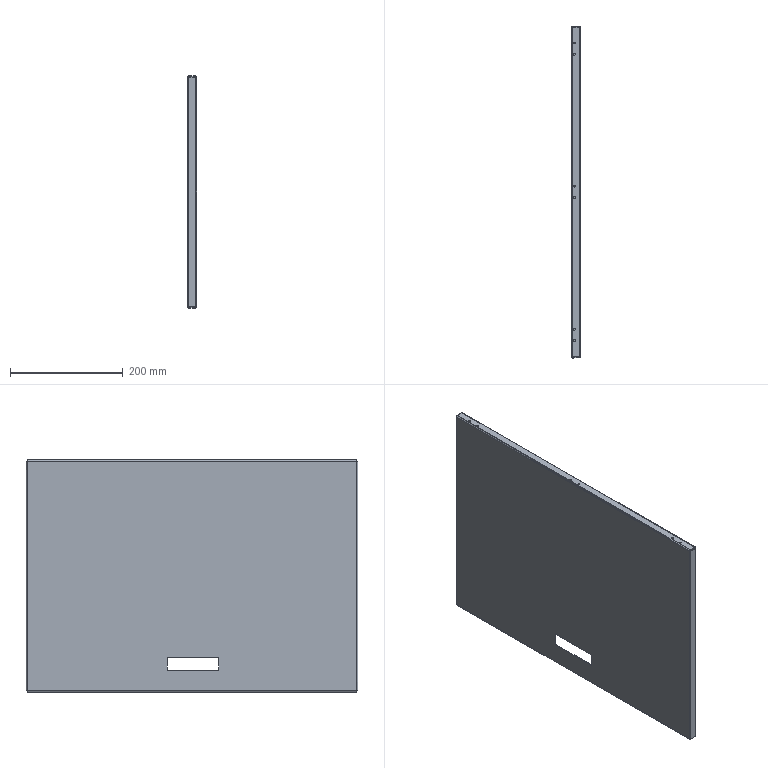Part | SolidWorks | features EdgeFlange 2, Cut 1, FlatPattern 1, HoleWzd 1, SMBaseFlange 1, SheetMetal 1 | 1 solid | 86 faces | box 16 x 588 x 411.5 mm | volume 451920 mm3 | plane 42 | cylinder 28 | spline 16 | commonest cylinder face diameters 3.3 x12 1.473 x8 4.473 x8